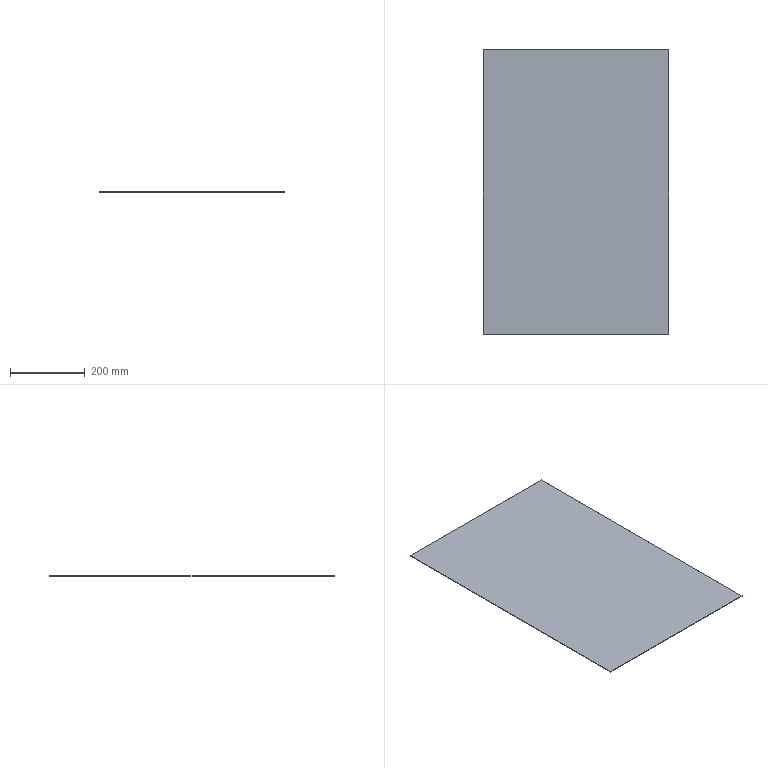Part | SolidWorks | 1 solid | 6 faces | box 496 x 760 x 1.5 mm | volume 565440 mm3 | plane 6
STEP:
#1=CARTESIAN_POINT('',(248.,-380.,0.));
#2=VERTEX_POINT('',#1);
#3=CARTESIAN_POINT('',(248.,380.,0.));
#4=VERTEX_POINT('',#3);
#5=CARTESIAN_POINT('',(248.,-380.,0.));
#6=DIRECTION('',(0.,1.,0.));
#7=VECTOR('',#6,1000.);
#8=LINE('',#5,#7);
#9=EDGE_CURVE('',#2,#4,#8,.T.);
#10=ORIENTED_EDGE('',*,*,#9,.T.);
#11=CARTESIAN_POINT('',(248.,380.,1.5));
#12=VERTEX_POINT('',#11);
#13=CARTESIAN_POINT('',(248.,380.,1.5));
#14=DIRECTION('',(0.,0.,-1.));
#15=VECTOR('',#14,1000.);
#16=LINE('',#13,#15);
#17=EDGE_CURVE('',#12,#4,#16,.T.);
#18=ORIENTED_EDGE('',*,*,#17,.F.);
#19=CARTESIAN_POINT('',(248.,-380.,1.5));
#20=VERTEX_POINT('',#19);
#21=CARTESIAN_POINT('',(248.,-380.,1.5));
#22=DIRECTION('',(0.,1.,0.));
#23=VECTOR('',#22,1000.);
#24=LINE('',#21,#23);
#25=EDGE_CURVE('',#20,#12,#24,.T.);
#26=ORIENTED_EDGE('',*,*,#25,.F.);
#27=CARTESIAN_POINT('',(248.,-380.,1.5));
#28=DIRECTION('',(0.,0.,-1.));
#29=VECTOR('',#28,1000.);
#30=LINE('',#27,#29);
#31=EDGE_CURVE('',#20,#2,#30,.T.);
#32=ORIENTED_EDGE('',*,*,#31,.T.);
#33=EDGE_LOOP('',(#10,#18,#26,#32));
#34=FACE_OUTER_BOUND('',#33,.T.);
#35=CARTESIAN_POINT('',(248.,-380.,1.5));
#36=DIRECTION('',(-1.,0.,0.));
#37=DIRECTION('',(0.,0.,1.));
#38=AXIS2_PLACEMENT_3D('',#35,#36,#37);
#39=PLANE('',#38);
#40=ADVANCED_FACE('',(#34),#39,.F.);
#41=CARTESIAN_POINT('',(-248.,380.,0.));
#42=VERTEX_POINT('',#41);
#43=CARTESIAN_POINT('',(248.,380.,0.));
#44=DIRECTION('',(-1.,0.,0.));
#45=VECTOR('',#44,1000.);
#46=LINE('',#43,#45);
#47=EDGE_CURVE('',#4,#42,#46,.T.);
#48=ORIENTED_EDGE('',*,*,#47,.T.);
#49=CARTESIAN_POINT('',(-248.,380.,1.5));
#50=VERTEX_POINT('',#49);
#51=CARTESIAN_POINT('',(-248.,380.,1.5));
#52=DIRECTION('',(0.,0.,-1.));
#53=VECTOR('',#52,1000.);
#54=LINE('',#51,#53);
#55=EDGE_CURVE('',#50,#42,#54,.T.);
#56=ORIENTED_EDGE('',*,*,#55,.F.);
#57=CARTESIAN_POINT('',(248.,380.,1.5));
#58=DIRECTION('',(-1.,0.,0.));
#59=VECTOR('',#58,1000.);
#60=LINE('',#57,#59);
#61=EDGE_CURVE('',#12,#50,#60,.T.);
#62=ORIENTED_EDGE('',*,*,#61,.F.);
#63=ORIENTED_EDGE('',*,*,#17,.T.);
#64=EDGE_LOOP('',(#48,#56,#62,#63));
#65=FACE_OUTER_BOUND('',#64,.T.);
#66=CARTESIAN_POINT('',(248.,380.,1.5));
#67=DIRECTION('',(0.,-1.,0.));
#68=DIRECTION('',(0.,0.,-1.));
#69=AXIS2_PLACEMENT_3D('',#66,#67,#68);
#70=PLANE('',#69);
#71=ADVANCED_FACE('',(#65),#70,.F.);
#72=CARTESIAN_POINT('',(-248.,-380.,0.));
#73=VERTEX_POINT('',#72);
#74=CARTESIAN_POINT('',(-248.,-380.,0.));
#75=DIRECTION('',(0.,-1.,0.));
#76=VECTOR('',#75,1000.);
#77=LINE('',#74,#76);
#78=EDGE_CURVE('',#42,#73,#77,.T.);
#79=ORIENTED_EDGE('',*,*,#78,.T.);
#80=CARTESIAN_POINT('',(-248.,-380.,1.5));
#81=VERTEX_POINT('',#80);
#82=CARTESIAN_POINT('',(-248.,-380.,1.5));
#83=DIRECTION('',(0.,0.,-1.));
#84=VECTOR('',#83,1000.);
#85=LINE('',#82,#84);
#86=EDGE_CURVE('',#81,#73,#85,.T.);
#87=ORIENTED_EDGE('',*,*,#86,.F.);
#88=CARTESIAN_POINT('',(-248.,-380.,1.5));
#89=DIRECTION('',(0.,-1.,0.));
#90=VECTOR('',#89,1000.);
#91=LINE('',#88,#90);
#92=EDGE_CURVE('',#50,#81,#91,.T.);
#93=ORIENTED_EDGE('',*,*,#92,.F.);
#94=ORIENTED_EDGE('',*,*,#55,.T.);
#95=EDGE_LOOP('',(#79,#87,#93,#94));
#96=FACE_OUTER_BOUND('',#95,.T.);
#97=CARTESIAN_POINT('',(-248.,-380.,1.5));
#98=DIRECTION('',(1.,0.,0.));
#99=DIRECTION('',(0.,0.,-1.));
#100=AXIS2_PLACEMENT_3D('',#97,#98,#99);
#101=PLANE('',#100);
#102=ADVANCED_FACE('',(#96),#101,.F.);
#103=CARTESIAN_POINT('',(248.,-380.,0.));
#104=DIRECTION('',(1.,0.,0.));
#105=VECTOR('',#104,1000.);
#106=LINE('',#103,#105);
#107=EDGE_CURVE('',#73,#2,#106,.T.);
#108=ORIENTED_EDGE('',*,*,#107,.T.);
#109=ORIENTED_EDGE('',*,*,#31,.F.);
#110=CARTESIAN_POINT('',(248.,-380.,1.5));
#111=DIRECTION('',(1.,0.,0.));
#112=VECTOR('',#111,1000.);
#113=LINE('',#110,#112);
#114=EDGE_CURVE('',#81,#20,#113,.T.);
#115=ORIENTED_EDGE('',*,*,#114,.F.);
#116=ORIENTED_EDGE('',*,*,#86,.T.);
#117=EDGE_LOOP('',(#108,#109,#115,#116));
#118=FACE_OUTER_BOUND('',#117,.T.);
#119=CARTESIAN_POINT('',(248.,-380.,1.5));
#120=DIRECTION('',(0.,1.,0.));
#121=DIRECTION('',(0.,0.,1.));
#122=AXIS2_PLACEMENT_3D('',#119,#120,#121);
#123=PLANE('',#122);
#124=ADVANCED_FACE('',(#118),#123,.F.);
#125=ORIENTED_EDGE('',*,*,#25,.T.);
#126=ORIENTED_EDGE('',*,*,#61,.T.);
#127=ORIENTED_EDGE('',*,*,#92,.T.);
#128=ORIENTED_EDGE('',*,*,#114,.T.);
#129=EDGE_LOOP('',(#125,#126,#127,#128));
#130=FACE_OUTER_BOUND('',#129,.T.);
#131=CARTESIAN_POINT('',(0.,0.,1.5));
#132=DIRECTION('',(0.,0.,1.));
#133=DIRECTION('',(1.,0.,0.));
#134=AXIS2_PLACEMENT_3D('',#131,#132,#133);
#135=PLANE('',#134);
#136=ADVANCED_FACE('',(#130),#135,.T.);
#137=ORIENTED_EDGE('',*,*,#9,.F.);
#138=ORIENTED_EDGE('',*,*,#107,.F.);
#139=ORIENTED_EDGE('',*,*,#78,.F.);
#140=ORIENTED_EDGE('',*,*,#47,.F.);
#141=EDGE_LOOP('',(#137,#138,#139,#140));
#142=FACE_OUTER_BOUND('',#141,.T.);
#143=CARTESIAN_POINT('',(0.,0.,0.));
#144=DIRECTION('',(0.,0.,1.));
#145=DIRECTION('',(1.,0.,0.));
#146=AXIS2_PLACEMENT_3D('',#143,#144,#145);
#147=PLANE('',#146);
#148=ADVANCED_FACE('',(#142),#147,.F.);
#149=CLOSED_SHELL('',(#40,#71,#102,#124,#136,#148));
#150=MANIFOLD_SOLID_BREP('',#149);
#151=CARTESIAN_POINT('',(0.,0.,0.));
#152=DIRECTION('',(0.,0.,1.));
#153=DIRECTION('',(1.,0.,0.));
#154=AXIS2_PLACEMENT_3D('',#151,#152,#153);
#155=(LENGTH_UNIT()NAMED_UNIT(*)SI_UNIT(.MILLI.,.METRE.));
#156=UNCERTAINTY_MEASURE_WITH_UNIT(LENGTH_MEASURE(0.00001),#155,'','');
#157=(NAMED_UNIT(*)PLANE_ANGLE_UNIT()SI_UNIT($,.RADIAN.));
#158=(NAMED_UNIT(*)SI_UNIT($,.STERADIAN.)SOLID_ANGLE_UNIT());
#159=(GEOMETRIC_REPRESENTATION_CONTEXT(3)GLOBAL_UNCERTAINTY_ASSIGNED_CONTEXT((#156))GLOBAL_UNIT_ASSIGNED_CONTEXT((#155,#157,#158))REPRESENTATION_CONTEXT('',''));
#160=ADVANCED_BREP_SHAPE_REPRESENTATION('',(#150,#154),#159);